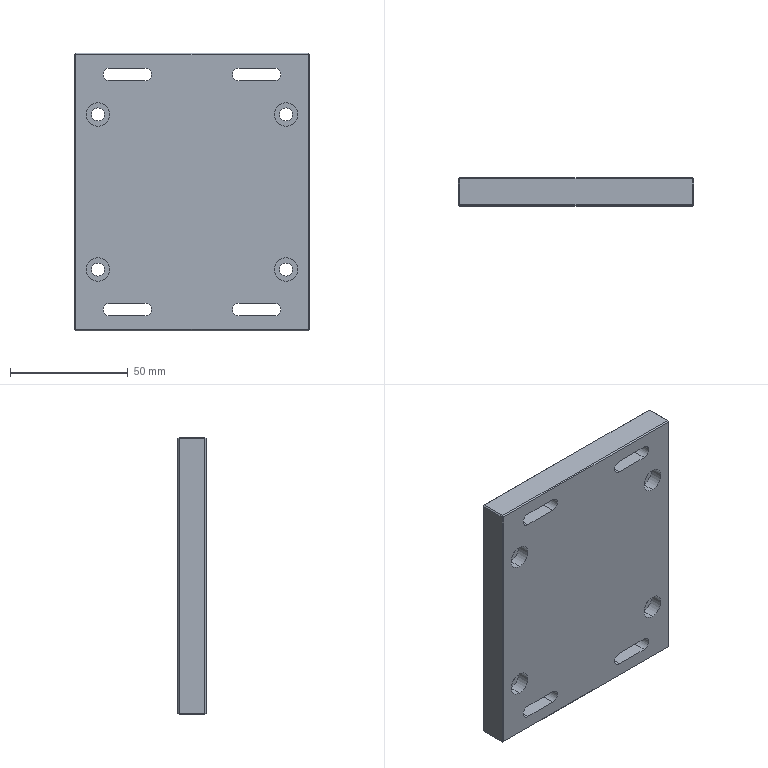Part | STEP file | ND25021-01-JDKM-18-TL | 1 solid | 68 faces | box 100 x 12 x 118 mm | volume 133882 mm3 | plane 38 | cylinder 26 | cone 4 | commonest cylinder face diameters 5.5 x16 10 x8 4.2 x2